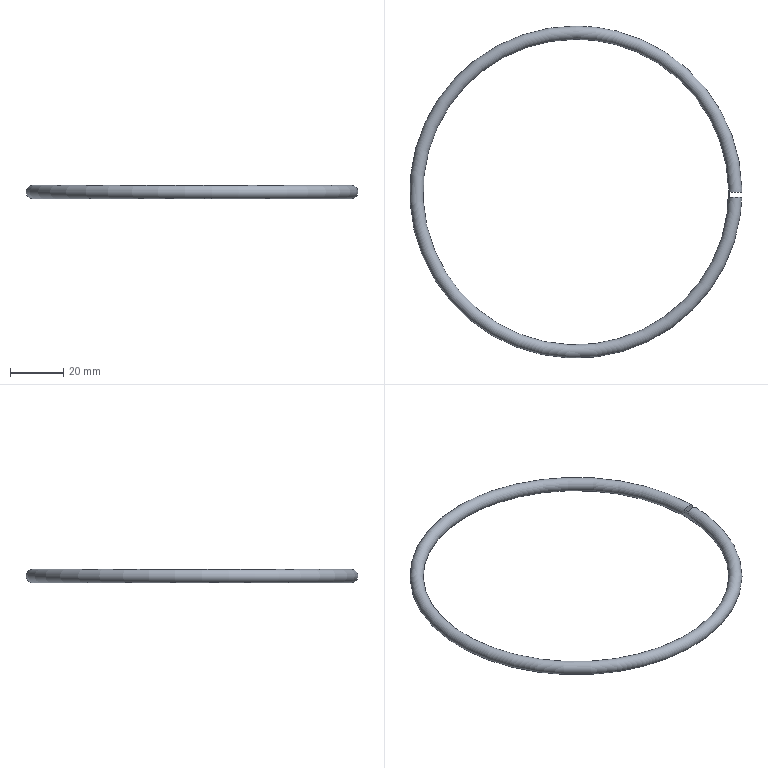Part | NX | features 1 2 | 1 solid | 4 faces | box 125.3 x 125.3 x 5 mm | volume 7384 mm3 | plane 3 | torus 1
STEP:
#1=CARTESIAN_POINT('',(2188.15,265.,28.));
#2=VERTEX_POINT('',#1);
#3=CARTESIAN_POINT('',(2188.15,265.,31.));
#4=VERTEX_POINT('',#3);
#5=CARTESIAN_POINT('',(2190.15,265.,29.5));
#6=DIRECTION('',(0.,-1.,0.));
#7=DIRECTION('',(1.,0.,0.));
#8=AXIS2_PLACEMENT_3D('',#5,#6,#7);
#9=CIRCLE('',#8,2.5);
#10=EDGE_CURVE('',#2,#4,#9,.T.);
#11=ORIENTED_EDGE('',*,*,#10,.F.);
#12=CARTESIAN_POINT('',(2188.15,263.,27.955));
#13=VERTEX_POINT('',#12);
#14=CARTESIAN_POINT('',(2188.15,263.,27.955));
#15=CARTESIAN_POINT('',(2188.15,263.666,27.984));
#16=CARTESIAN_POINT('',(2188.15,264.333,28.));
#17=CARTESIAN_POINT('',(2188.15,265.,28.));
#18=B_SPLINE_CURVE_WITH_KNOTS('',3,(#14,#15,#16,#17),.UNSPECIFIED.,.F.,.F.,(4,4),(0.,0.002001),.UNSPECIFIED.);
#19=EDGE_CURVE('',#13,#2,#18,.T.);
#20=ORIENTED_EDGE('',*,*,#19,.F.);
#21=CARTESIAN_POINT('',(2188.15,263.,31.045));
#22=VERTEX_POINT('',#21);
#23=CARTESIAN_POINT('',(2188.15,263.,31.045));
#24=CARTESIAN_POINT('',(2188.794,263.,31.863));
#25=CARTESIAN_POINT('',(2190.547,263.,32.354));
#26=CARTESIAN_POINT('',(2192.289,263.,31.045));
#27=CARTESIAN_POINT('',(2192.783,263.,29.501));
#28=CARTESIAN_POINT('',(2192.289,263.,27.957));
#29=CARTESIAN_POINT('',(2190.553,263.,26.647));
#30=CARTESIAN_POINT('',(2188.794,263.,27.137));
#31=CARTESIAN_POINT('',(2188.15,263.,27.955));
#32=B_SPLINE_CURVE_WITH_KNOTS('',3,(#23,#24,#25,#26,#27,#28,#29,#30,#31),.UNSPECIFIED.,.F.,.F.,(4,1,1,1,1,1,4),(0.,0.00308,0.00462,0.00616,0.0077,0.00924,0.01232),.UNSPECIFIED.);
#33=EDGE_CURVE('',#22,#13,#32,.T.);
#34=ORIENTED_EDGE('',*,*,#33,.F.);
#35=CARTESIAN_POINT('',(2188.15,265.,31.));
#36=CARTESIAN_POINT('',(2188.15,264.333,31.));
#37=CARTESIAN_POINT('',(2188.15,263.666,31.016));
#38=CARTESIAN_POINT('',(2188.15,263.,31.045));
#39=B_SPLINE_CURVE_WITH_KNOTS('',3,(#35,#36,#37,#38),.UNSPECIFIED.,.F.,.F.,(4,4),(0.,0.002001),.UNSPECIFIED.);
#40=EDGE_CURVE('',#4,#22,#39,.T.);
#41=ORIENTED_EDGE('',*,*,#40,.F.);
#42=EDGE_LOOP('',(#11,#20,#34,#41));
#43=FACE_BOUND('',#42,.T.);
#44=CARTESIAN_POINT('',(2130.,265.,29.5));
#45=DIRECTION('',(0.,0.,1.));
#46=DIRECTION('',(-1.,0.,0.));
#47=AXIS2_PLACEMENT_3D('',#44,#45,#46);
#48=TOROIDAL_SURFACE('',#47,60.15,2.5);
#49=ADVANCED_FACE('',(#43),#48,.T.);
#50=ORIENTED_EDGE('',*,*,#33,.T.);
#51=CARTESIAN_POINT('',(2188.15,263.,24.5));
#52=DIRECTION('',(0.,0.,1.));
#53=VECTOR('',#52,1000.);
#54=LINE('',#51,#53);
#55=EDGE_CURVE('',#13,#22,#54,.T.);
#56=ORIENTED_EDGE('',*,*,#55,.T.);
#57=EDGE_LOOP('',(#50,#56));
#58=FACE_BOUND('',#57,.T.);
#59=CARTESIAN_POINT('',(2188.15,263.,24.5));
#60=DIRECTION('',(0.,-1.,0.));
#61=DIRECTION('',(0.,0.,1.));
#62=AXIS2_PLACEMENT_3D('',#59,#60,#61);
#63=PLANE('',#62);
#64=ADVANCED_FACE('',(#58),#63,.F.);
#65=ORIENTED_EDGE('',*,*,#10,.T.);
#66=CARTESIAN_POINT('',(2188.15,265.,24.5));
#67=DIRECTION('',(0.,0.,1.));
#68=VECTOR('',#67,1000.);
#69=LINE('',#66,#68);
#70=EDGE_CURVE('',#2,#4,#69,.T.);
#71=ORIENTED_EDGE('',*,*,#70,.F.);
#72=EDGE_LOOP('',(#65,#71));
#73=FACE_BOUND('',#72,.T.);
#74=CARTESIAN_POINT('',(2193.15,265.,24.5));
#75=DIRECTION('',(0.,1.,0.));
#76=DIRECTION('',(0.,0.,-1.));
#77=AXIS2_PLACEMENT_3D('',#74,#75,#76);
#78=PLANE('',#77);
#79=ADVANCED_FACE('',(#73),#78,.F.);
#80=ORIENTED_EDGE('',*,*,#40,.T.);
#81=ORIENTED_EDGE('',*,*,#55,.F.);
#82=ORIENTED_EDGE('',*,*,#19,.T.);
#83=ORIENTED_EDGE('',*,*,#70,.T.);
#84=EDGE_LOOP('',(#80,#81,#82,#83));
#85=FACE_BOUND('',#84,.T.);
#86=CARTESIAN_POINT('',(2188.15,265.,24.5));
#87=DIRECTION('',(-1.,0.,0.));
#88=DIRECTION('',(0.,0.,-1.));
#89=AXIS2_PLACEMENT_3D('',#86,#87,#88);
#90=PLANE('',#89);
#91=ADVANCED_FACE('',(#85),#90,.F.);
#92=CLOSED_SHELL('',(#49,#64,#79,#91));
#93=MANIFOLD_SOLID_BREP('',#92);
#94=(LENGTH_UNIT()NAMED_UNIT(*)SI_UNIT(.MILLI.,.METRE.));
#95=UNCERTAINTY_MEASURE_WITH_UNIT(LENGTH_MEASURE(0.0508),#94,'','');
#96=(NAMED_UNIT(*)PLANE_ANGLE_UNIT()SI_UNIT($,.RADIAN.));
#97=(NAMED_UNIT(*)SI_UNIT($,.STERADIAN.)SOLID_ANGLE_UNIT());
#98=(GEOMETRIC_REPRESENTATION_CONTEXT(3)GLOBAL_UNCERTAINTY_ASSIGNED_CONTEXT((#95))GLOBAL_UNIT_ASSIGNED_CONTEXT((#94,#96,#97))REPRESENTATION_CONTEXT('',''));
#99=ADVANCED_BREP_SHAPE_REPRESENTATION('',(#93),#98);